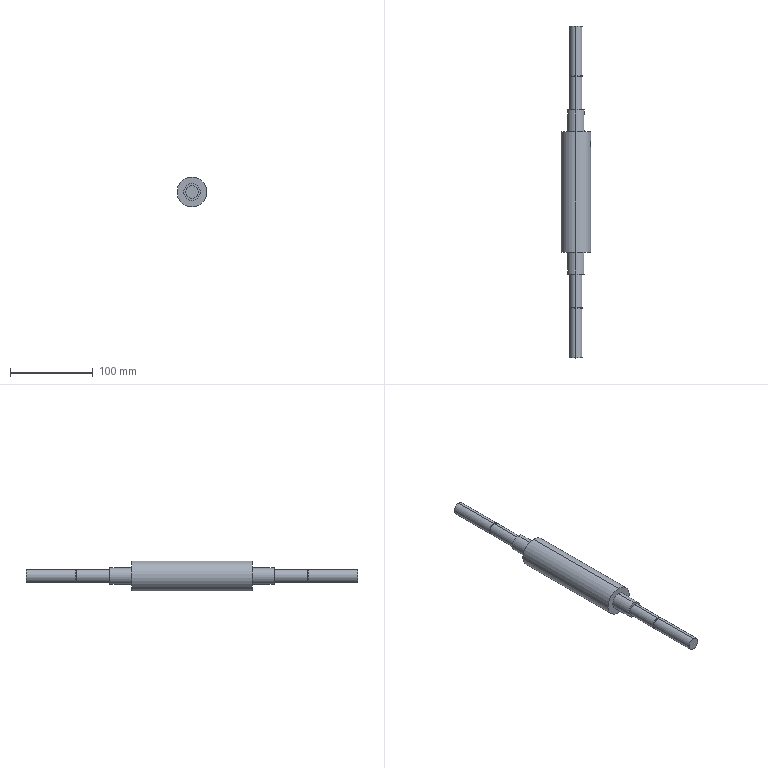Part | STEP file | 1 solid | 37 faces | box 36 x 400 x 36 mm | volume 199320 mm3 | cylinder 23 | plane 14 | commonest cylinder face diameters 15 x8 13 x4 20 x4 6 x3 10 x2 36 x2